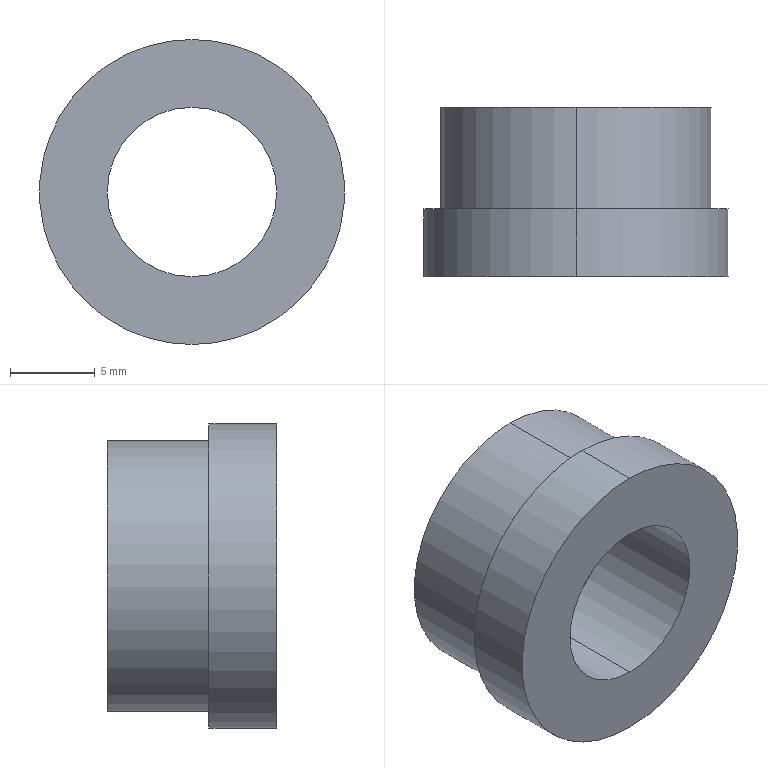Part | SolidWorks | features ICE 2, Chamfer 1, Extrusion 1 | 1 solid | 10 faces | box 18 x 10 x 18 mm | volume 1269 mm3 | cylinder 6 | cone 2 | plane 2 | commonest cylinder face diameters 10 x2 16 x2 18 x2
STEP:
#1=CARTESIAN_POINT('',(0.,7.,-5.));
#2=VERTEX_POINT('',#1);
#3=CARTESIAN_POINT('',(0.,7.,5.));
#4=VERTEX_POINT('',#3);
#5=CARTESIAN_POINT('',(0.,7.,0.));
#6=DIRECTION('',(0.,1.,0.));
#7=DIRECTION('',(0.,0.,1.));
#8=AXIS2_PLACEMENT_3D('',#5,#6,#7);
#9=CIRCLE('',#8,5.);
#10=EDGE_CURVE('',#2,#4,#9,.T.);
#11=ORIENTED_EDGE('',*,*,#10,.F.);
#12=CARTESIAN_POINT('',(0.,10.,-8.));
#13=VERTEX_POINT('',#12);
#14=CARTESIAN_POINT('',(0.,7.,-5.));
#15=DIRECTION('',(0.,0.7071,-0.7071));
#16=VECTOR('',#15,1000.);
#17=LINE('',#14,#16);
#18=EDGE_CURVE('',#2,#13,#17,.T.);
#19=ORIENTED_EDGE('',*,*,#18,.T.);
#20=CARTESIAN_POINT('',(0.,10.,8.));
#21=VERTEX_POINT('',#20);
#22=CARTESIAN_POINT('',(0.,10.,0.));
#23=DIRECTION('',(0.,1.,0.));
#24=DIRECTION('',(0.,0.,1.));
#25=AXIS2_PLACEMENT_3D('',#22,#23,#24);
#26=CIRCLE('',#25,8.);
#27=EDGE_CURVE('',#13,#21,#26,.T.);
#28=ORIENTED_EDGE('',*,*,#27,.T.);
#29=CARTESIAN_POINT('',(0.,7.,5.));
#30=DIRECTION('',(0.,0.7071,0.7071));
#31=VECTOR('',#30,1000.);
#32=LINE('',#29,#31);
#33=EDGE_CURVE('',#4,#21,#32,.T.);
#34=ORIENTED_EDGE('',*,*,#33,.F.);
#35=EDGE_LOOP('',(#11,#19,#28,#34));
#36=FACE_OUTER_BOUND('',#35,.T.);
#37=CARTESIAN_POINT('',(0.,7.,0.));
#38=DIRECTION('',(0.,1.,0.));
#39=DIRECTION('',(0.,0.,1.));
#40=AXIS2_PLACEMENT_3D('',#37,#38,#39);
#41=CONICAL_SURFACE('',#40,5.,0.7854);
#42=ADVANCED_FACE('',(#36),#41,.F.);
#43=CARTESIAN_POINT('',(0.,0.,-5.));
#44=VERTEX_POINT('',#43);
#45=CARTESIAN_POINT('',(0.,0.,5.));
#46=VERTEX_POINT('',#45);
#47=CARTESIAN_POINT('',(0.,0.,0.));
#48=DIRECTION('',(0.,1.,0.));
#49=DIRECTION('',(0.,0.,1.));
#50=AXIS2_PLACEMENT_3D('',#47,#48,#49);
#51=CIRCLE('',#50,5.);
#52=EDGE_CURVE('',#44,#46,#51,.T.);
#53=ORIENTED_EDGE('',*,*,#52,.F.);
#54=CARTESIAN_POINT('',(0.,-40.,-5.));
#55=DIRECTION('',(0.,1.,0.));
#56=VECTOR('',#55,1000.);
#57=LINE('',#54,#56);
#58=EDGE_CURVE('',#44,#2,#57,.T.);
#59=ORIENTED_EDGE('',*,*,#58,.T.);
#60=ORIENTED_EDGE('',*,*,#10,.T.);
#61=CARTESIAN_POINT('',(0.,-40.,5.));
#62=DIRECTION('',(0.,1.,0.));
#63=VECTOR('',#62,1000.);
#64=LINE('',#61,#63);
#65=EDGE_CURVE('',#46,#4,#64,.T.);
#66=ORIENTED_EDGE('',*,*,#65,.F.);
#67=EDGE_LOOP('',(#53,#59,#60,#66));
#68=FACE_OUTER_BOUND('',#67,.T.);
#69=CARTESIAN_POINT('',(0.,-40.,0.));
#70=DIRECTION('',(0.,1.,0.));
#71=DIRECTION('',(0.,0.,1.));
#72=AXIS2_PLACEMENT_3D('',#69,#70,#71);
#73=CYLINDRICAL_SURFACE('',#72,5.);
#74=ADVANCED_FACE('',(#68),#73,.F.);
#75=CARTESIAN_POINT('',(0.,10.,0.));
#76=DIRECTION('',(0.,1.,0.));
#77=DIRECTION('',(0.,0.,1.));
#78=AXIS2_PLACEMENT_3D('',#75,#76,#77);
#79=CIRCLE('',#78,8.);
#80=EDGE_CURVE('',#21,#13,#79,.T.);
#81=ORIENTED_EDGE('',*,*,#80,.F.);
#82=CARTESIAN_POINT('',(0.,4.,8.));
#83=VERTEX_POINT('',#82);
#84=CARTESIAN_POINT('',(0.,10.,8.));
#85=DIRECTION('',(0.,-1.,0.));
#86=VECTOR('',#85,1000.);
#87=LINE('',#84,#86);
#88=EDGE_CURVE('',#21,#83,#87,.T.);
#89=ORIENTED_EDGE('',*,*,#88,.T.);
#90=CARTESIAN_POINT('',(0.,4.,-8.));
#91=VERTEX_POINT('',#90);
#92=CARTESIAN_POINT('',(0.,4.,0.));
#93=DIRECTION('',(0.,1.,0.));
#94=DIRECTION('',(0.,0.,1.));
#95=AXIS2_PLACEMENT_3D('',#92,#93,#94);
#96=CIRCLE('',#95,8.);
#97=EDGE_CURVE('',#83,#91,#96,.T.);
#98=ORIENTED_EDGE('',*,*,#97,.T.);
#99=CARTESIAN_POINT('',(0.,10.,-8.));
#100=DIRECTION('',(0.,-1.,0.));
#101=VECTOR('',#100,1000.);
#102=LINE('',#99,#101);
#103=EDGE_CURVE('',#13,#91,#102,.T.);
#104=ORIENTED_EDGE('',*,*,#103,.F.);
#105=EDGE_LOOP('',(#81,#89,#98,#104));
#106=FACE_OUTER_BOUND('',#105,.T.);
#107=CARTESIAN_POINT('',(0.,10.,0.));
#108=DIRECTION('',(0.,-1.,0.));
#109=DIRECTION('',(0.,0.,-1.));
#110=AXIS2_PLACEMENT_3D('',#107,#108,#109);
#111=CYLINDRICAL_SURFACE('',#110,8.);
#112=ADVANCED_FACE('',(#106),#111,.T.);
#113=CARTESIAN_POINT('',(0.,4.,9.));
#114=VERTEX_POINT('',#113);
#115=CARTESIAN_POINT('',(0.,4.,-9.));
#116=VERTEX_POINT('',#115);
#117=CARTESIAN_POINT('',(0.,4.,0.));
#118=DIRECTION('',(0.,1.,0.));
#119=DIRECTION('',(0.,0.,1.));
#120=AXIS2_PLACEMENT_3D('',#117,#118,#119);
#121=CIRCLE('',#120,9.);
#122=EDGE_CURVE('',#114,#116,#121,.T.);
#123=ORIENTED_EDGE('',*,*,#122,.F.);
#124=CARTESIAN_POINT('',(0.,0.,9.));
#125=VERTEX_POINT('',#124);
#126=CARTESIAN_POINT('',(0.,4.,9.));
#127=DIRECTION('',(0.,-1.,0.));
#128=VECTOR('',#127,1000.);
#129=LINE('',#126,#128);
#130=EDGE_CURVE('',#114,#125,#129,.T.);
#131=ORIENTED_EDGE('',*,*,#130,.T.);
#132=CARTESIAN_POINT('',(0.,0.,-9.));
#133=VERTEX_POINT('',#132);
#134=CARTESIAN_POINT('',(0.,0.,0.));
#135=DIRECTION('',(0.,1.,0.));
#136=DIRECTION('',(0.,0.,1.));
#137=AXIS2_PLACEMENT_3D('',#134,#135,#136);
#138=CIRCLE('',#137,9.);
#139=EDGE_CURVE('',#125,#133,#138,.T.);
#140=ORIENTED_EDGE('',*,*,#139,.T.);
#141=CARTESIAN_POINT('',(0.,4.,-9.));
#142=DIRECTION('',(0.,-1.,0.));
#143=VECTOR('',#142,1000.);
#144=LINE('',#141,#143);
#145=EDGE_CURVE('',#116,#133,#144,.T.);
#146=ORIENTED_EDGE('',*,*,#145,.F.);
#147=EDGE_LOOP('',(#123,#131,#140,#146));
#148=FACE_OUTER_BOUND('',#147,.T.);
#149=CARTESIAN_POINT('',(0.,4.,0.));
#150=DIRECTION('',(0.,-1.,0.));
#151=DIRECTION('',(0.,0.,-1.));
#152=AXIS2_PLACEMENT_3D('',#149,#150,#151);
#153=CYLINDRICAL_SURFACE('',#152,9.);
#154=ADVANCED_FACE('',(#148),#153,.T.);
#155=ORIENTED_EDGE('',*,*,#130,.F.);
#156=CARTESIAN_POINT('',(0.,4.,0.));
#157=DIRECTION('',(0.,1.,0.));
#158=DIRECTION('',(0.,0.,1.));
#159=AXIS2_PLACEMENT_3D('',#156,#157,#158);
#160=CIRCLE('',#159,9.);
#161=EDGE_CURVE('',#116,#114,#160,.T.);
#162=ORIENTED_EDGE('',*,*,#161,.F.);
#163=ORIENTED_EDGE('',*,*,#145,.T.);
#164=CARTESIAN_POINT('',(0.,0.,0.));
#165=DIRECTION('',(0.,1.,0.));
#166=DIRECTION('',(0.,0.,1.));
#167=AXIS2_PLACEMENT_3D('',#164,#165,#166);
#168=CIRCLE('',#167,9.);
#169=EDGE_CURVE('',#133,#125,#168,.T.);
#170=ORIENTED_EDGE('',*,*,#169,.T.);
#171=EDGE_LOOP('',(#155,#162,#163,#170));
#172=FACE_OUTER_BOUND('',#171,.T.);
#173=CARTESIAN_POINT('',(0.,4.,0.));
#174=DIRECTION('',(0.,-1.,0.));
#175=DIRECTION('',(0.,0.,-1.));
#176=AXIS2_PLACEMENT_3D('',#173,#174,#175);
#177=CYLINDRICAL_SURFACE('',#176,9.);
#178=ADVANCED_FACE('',(#172),#177,.T.);
#179=CARTESIAN_POINT('',(0.,4.,0.));
#180=DIRECTION('',(0.,1.,0.));
#181=DIRECTION('',(0.,0.,1.));
#182=AXIS2_PLACEMENT_3D('',#179,#180,#181);
#183=CIRCLE('',#182,8.);
#184=EDGE_CURVE('',#91,#83,#183,.T.);
#185=ORIENTED_EDGE('',*,*,#184,.F.);
#186=ORIENTED_EDGE('',*,*,#97,.F.);
#187=EDGE_LOOP('',(#185,#186));
#188=FACE_BOUND('',#187,.T.);
#189=ORIENTED_EDGE('',*,*,#161,.T.);
#190=ORIENTED_EDGE('',*,*,#122,.T.);
#191=EDGE_LOOP('',(#189,#190));
#192=FACE_OUTER_BOUND('',#191,.T.);
#193=CARTESIAN_POINT('',(0.,4.,0.));
#194=DIRECTION('',(0.,1.,0.));
#195=DIRECTION('',(0.,0.,1.));
#196=AXIS2_PLACEMENT_3D('',#193,#194,#195);
#197=PLANE('',#196);
#198=ADVANCED_FACE('',(#188,#192),#197,.T.);
#199=CARTESIAN_POINT('',(0.,0.,0.));
#200=DIRECTION('',(0.,1.,0.));
#201=DIRECTION('',(0.,0.,1.));
#202=AXIS2_PLACEMENT_3D('',#199,#200,#201);
#203=CIRCLE('',#202,5.);
#204=EDGE_CURVE('',#46,#44,#203,.T.);
#205=ORIENTED_EDGE('',*,*,#204,.T.);
#206=ORIENTED_EDGE('',*,*,#52,.T.);
#207=EDGE_LOOP('',(#205,#206));
#208=FACE_BOUND('',#207,.T.);
#209=ORIENTED_EDGE('',*,*,#169,.F.);
#210=ORIENTED_EDGE('',*,*,#139,.F.);
#211=EDGE_LOOP('',(#209,#210));
#212=FACE_OUTER_BOUND('',#211,.T.);
#213=CARTESIAN_POINT('',(0.,0.,0.));
#214=DIRECTION('',(0.,1.,0.));
#215=DIRECTION('',(0.,0.,1.));
#216=AXIS2_PLACEMENT_3D('',#213,#214,#215);
#217=PLANE('',#216);
#218=ADVANCED_FACE('',(#208,#212),#217,.F.);
#219=ORIENTED_EDGE('',*,*,#88,.F.);
#220=ORIENTED_EDGE('',*,*,#27,.F.);
#221=ORIENTED_EDGE('',*,*,#103,.T.);
#222=ORIENTED_EDGE('',*,*,#184,.T.);
#223=EDGE_LOOP('',(#219,#220,#221,#222));
#224=FACE_OUTER_BOUND('',#223,.T.);
#225=CARTESIAN_POINT('',(0.,10.,0.));
#226=DIRECTION('',(0.,-1.,0.));
#227=DIRECTION('',(0.,0.,-1.));
#228=AXIS2_PLACEMENT_3D('',#225,#226,#227);
#229=CYLINDRICAL_SURFACE('',#228,8.);
#230=ADVANCED_FACE('',(#224),#229,.T.);
#231=ORIENTED_EDGE('',*,*,#58,.F.);
#232=ORIENTED_EDGE('',*,*,#204,.F.);
#233=ORIENTED_EDGE('',*,*,#65,.T.);
#234=CARTESIAN_POINT('',(0.,7.,0.));
#235=DIRECTION('',(0.,1.,0.));
#236=DIRECTION('',(0.,0.,1.));
#237=AXIS2_PLACEMENT_3D('',#234,#235,#236);
#238=CIRCLE('',#237,5.);
#239=EDGE_CURVE('',#4,#2,#238,.T.);
#240=ORIENTED_EDGE('',*,*,#239,.T.);
#241=EDGE_LOOP('',(#231,#232,#233,#240));
#242=FACE_OUTER_BOUND('',#241,.T.);
#243=CARTESIAN_POINT('',(0.,-40.,0.));
#244=DIRECTION('',(0.,1.,0.));
#245=DIRECTION('',(0.,0.,1.));
#246=AXIS2_PLACEMENT_3D('',#243,#244,#245);
#247=CYLINDRICAL_SURFACE('',#246,5.);
#248=ADVANCED_FACE('',(#242),#247,.F.);
#249=ORIENTED_EDGE('',*,*,#18,.F.);
#250=ORIENTED_EDGE('',*,*,#239,.F.);
#251=ORIENTED_EDGE('',*,*,#33,.T.);
#252=ORIENTED_EDGE('',*,*,#80,.T.);
#253=EDGE_LOOP('',(#249,#250,#251,#252));
#254=FACE_OUTER_BOUND('',#253,.T.);
#255=CARTESIAN_POINT('',(0.,7.,0.));
#256=DIRECTION('',(0.,1.,0.));
#257=DIRECTION('',(0.,0.,1.));
#258=AXIS2_PLACEMENT_3D('',#255,#256,#257);
#259=CONICAL_SURFACE('',#258,5.,0.7854);
#260=ADVANCED_FACE('',(#254),#259,.F.);
#261=CLOSED_SHELL('',(#42,#74,#112,#154,#178,#198,#218,#230,#248,#260));
#262=MANIFOLD_SOLID_BREP('',#261);
#263=CARTESIAN_POINT('',(0.,0.,0.));
#264=DIRECTION('',(0.,0.,1.));
#265=DIRECTION('',(1.,0.,0.));
#266=AXIS2_PLACEMENT_3D('',#263,#264,#265);
#267=(LENGTH_UNIT()NAMED_UNIT(*)SI_UNIT(.MILLI.,.METRE.));
#268=UNCERTAINTY_MEASURE_WITH_UNIT(LENGTH_MEASURE(0.00001),#267,'','');
#269=(NAMED_UNIT(*)PLANE_ANGLE_UNIT()SI_UNIT($,.RADIAN.));
#270=(NAMED_UNIT(*)SI_UNIT($,.STERADIAN.)SOLID_ANGLE_UNIT());
#271=(GEOMETRIC_REPRESENTATION_CONTEXT(3)GLOBAL_UNCERTAINTY_ASSIGNED_CONTEXT((#268))GLOBAL_UNIT_ASSIGNED_CONTEXT((#267,#269,#270))REPRESENTATION_CONTEXT('',''));
#272=ADVANCED_BREP_SHAPE_REPRESENTATION('',(#262,#266),#271);